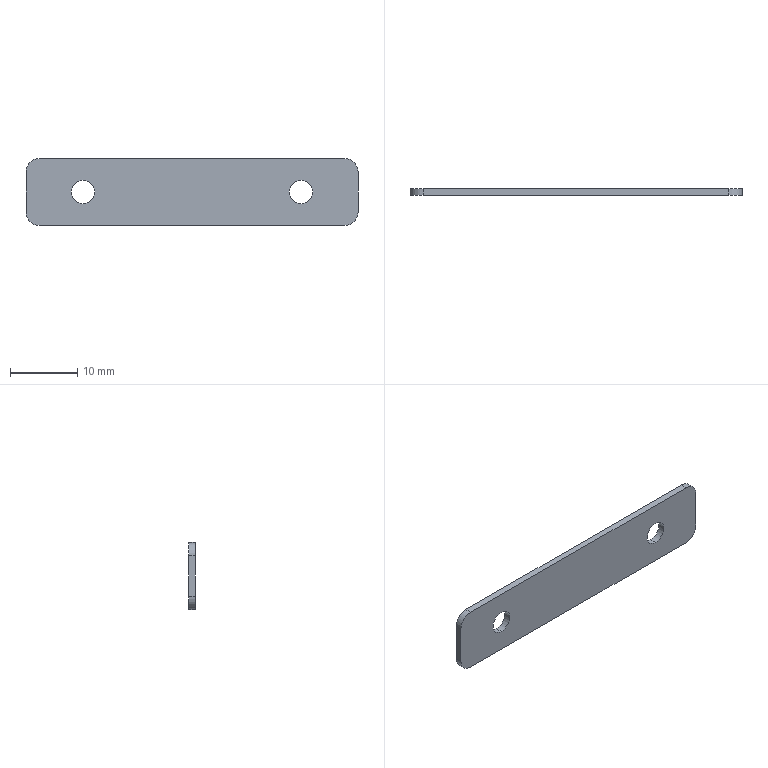Part | STEP file | 1 solid | 14 faces | box 49.5 x 1 x 10 mm | volume 472.324 mm3 | cylinder 8 | plane 6 | commonest cylinder face diameters 3.5 x4 4 x4
STEP:
#1=CARTESIAN_POINT('',(0.,0.,0.));
#2=DIRECTION('',(0.,0.,1.));
#3=DIRECTION('',(1.,0.,0.));
#4=AXIS2_PLACEMENT_3D('',#1,#2,#3);
#5=CARTESIAN_POINT('',(-16.25,1.,-1.75));
#6=VERTEX_POINT('',#5);
#7=CARTESIAN_POINT('',(-16.25,0.,-1.75));
#8=VERTEX_POINT('',#7);
#9=CARTESIAN_POINT('',(-16.25,1.,-1.75));
#10=DIRECTION('',(0.,-1.,0.));
#11=VECTOR('',#10,1.);
#12=LINE('',#9,#11);
#13=CARTESIAN_POINT('',(-16.25,1.,0.));
#14=DIRECTION('',(0.,-1.,0.));
#15=DIRECTION('',(0.,0.,-1.));
#16=AXIS2_PLACEMENT_3D('',#13,#14,#15);
#17=CYLINDRICAL_SURFACE('',#16,1.75);
#18=CARTESIAN_POINT('',(6.283,0.));
#19=DIRECTION('',(0.,1.));
#20=VECTOR('',#19,1.);
#21=LINE('',#18,#20);
#22=(GEOMETRIC_REPRESENTATION_CONTEXT(2)PARAMETRIC_REPRESENTATION_CONTEXT()REPRESENTATION_CONTEXT('',''));
#23=DEFINITIONAL_REPRESENTATION('',(#21),#22);
#24=PCURVE('',#17,#23);
#25=CARTESIAN_POINT('',(-16.25,1.,0.));
#26=DIRECTION('',(0.,-1.,0.));
#27=DIRECTION('',(0.,0.,-1.));
#28=AXIS2_PLACEMENT_3D('',#25,#26,#27);
#29=CYLINDRICAL_SURFACE('',#28,1.75);
#30=CARTESIAN_POINT('',(0.,0.));
#31=DIRECTION('',(0.,1.));
#32=VECTOR('',#31,1.);
#33=LINE('',#30,#32);
#34=(GEOMETRIC_REPRESENTATION_CONTEXT(2)PARAMETRIC_REPRESENTATION_CONTEXT()REPRESENTATION_CONTEXT('',''));
#35=DEFINITIONAL_REPRESENTATION('',(#33),#34);
#36=PCURVE('',#29,#35);
#37=SURFACE_CURVE('',#12,(#24,#36),.PCURVE_S1.);
#38=EDGE_CURVE('',#6,#8,#37,.T.);
#39=ORIENTED_EDGE('',*,*,#38,.T.);
#40=CARTESIAN_POINT('',(-16.25,0.,1.75));
#41=VERTEX_POINT('',#40);
#42=CARTESIAN_POINT('',(-16.25,0.,0.));
#43=DIRECTION('',(0.,1.,0.));
#44=DIRECTION('',(0.,0.,-1.));
#45=AXIS2_PLACEMENT_3D('',#42,#43,#44);
#46=CIRCLE('',#45,1.75);
#47=CARTESIAN_POINT('',(6.283,1.));
#48=DIRECTION('',(-1.,0.));
#49=VECTOR('',#48,1.);
#50=LINE('',#47,#49);
#51=(GEOMETRIC_REPRESENTATION_CONTEXT(2)PARAMETRIC_REPRESENTATION_CONTEXT()REPRESENTATION_CONTEXT('',''));
#52=DEFINITIONAL_REPRESENTATION('',(#50),#51);
#53=PCURVE('',#17,#52);
#54=CARTESIAN_POINT('',(0.,0.,0.));
#55=DIRECTION('',(0.,1.,0.));
#56=DIRECTION('',(1.,0.,0.));
#57=AXIS2_PLACEMENT_3D('',#54,#55,#56);
#58=PLANE('',#57);
#59=CARTESIAN_POINT('',(-16.25,0.));
#60=DIRECTION('',(0.,1.));
#61=AXIS2_PLACEMENT_2D('',#59,#60);
#62=CIRCLE('',#61,1.75);
#63=(GEOMETRIC_REPRESENTATION_CONTEXT(2)PARAMETRIC_REPRESENTATION_CONTEXT()REPRESENTATION_CONTEXT('',''));
#64=DEFINITIONAL_REPRESENTATION('',(#62),#63);
#65=PCURVE('',#58,#64);
#66=SURFACE_CURVE('',#46,(#53,#65),.PCURVE_S1.);
#67=EDGE_CURVE('',#8,#41,#66,.T.);
#68=ORIENTED_EDGE('',*,*,#67,.T.);
#69=CARTESIAN_POINT('',(-16.25,1.,1.75));
#70=VERTEX_POINT('',#69);
#71=CARTESIAN_POINT('',(-16.25,1.,1.75));
#72=DIRECTION('',(0.,-1.,0.));
#73=VECTOR('',#72,1.);
#74=LINE('',#71,#73);
#75=CARTESIAN_POINT('',(3.142,0.));
#76=DIRECTION('',(0.,1.));
#77=VECTOR('',#76,1.);
#78=LINE('',#75,#77);
#79=(GEOMETRIC_REPRESENTATION_CONTEXT(2)PARAMETRIC_REPRESENTATION_CONTEXT()REPRESENTATION_CONTEXT('',''));
#80=DEFINITIONAL_REPRESENTATION('',(#78),#79);
#81=PCURVE('',#17,#80);
#82=CARTESIAN_POINT('',(3.142,0.));
#83=DIRECTION('',(0.,1.));
#84=VECTOR('',#83,1.);
#85=LINE('',#82,#84);
#86=(GEOMETRIC_REPRESENTATION_CONTEXT(2)PARAMETRIC_REPRESENTATION_CONTEXT()REPRESENTATION_CONTEXT('',''));
#87=DEFINITIONAL_REPRESENTATION('',(#85),#86);
#88=PCURVE('',#29,#87);
#89=SURFACE_CURVE('',#74,(#81,#88),.PCURVE_S1.);
#90=EDGE_CURVE('',#70,#41,#89,.T.);
#91=ORIENTED_EDGE('',*,*,#90,.F.);
#92=CARTESIAN_POINT('',(-16.25,1.,0.));
#93=DIRECTION('',(0.,-1.,0.));
#94=DIRECTION('',(0.,0.,-1.));
#95=AXIS2_PLACEMENT_3D('',#92,#93,#94);
#96=CIRCLE('',#95,1.75);
#97=CARTESIAN_POINT('',(0.,0.));
#98=DIRECTION('',(1.,0.));
#99=VECTOR('',#98,1.);
#100=LINE('',#97,#99);
#101=(GEOMETRIC_REPRESENTATION_CONTEXT(2)PARAMETRIC_REPRESENTATION_CONTEXT()REPRESENTATION_CONTEXT('',''));
#102=DEFINITIONAL_REPRESENTATION('',(#100),#101);
#103=PCURVE('',#17,#102);
#104=CARTESIAN_POINT('',(0.,1.,0.));
#105=DIRECTION('',(0.,1.,0.));
#106=DIRECTION('',(1.,0.,0.));
#107=AXIS2_PLACEMENT_3D('',#104,#105,#106);
#108=PLANE('',#107);
#109=CARTESIAN_POINT('',(-16.25,1.75));
#110=CARTESIAN_POINT('',(-13.219,1.75));
#111=CARTESIAN_POINT('',(-14.734,-0.875));
#112=CARTESIAN_POINT('',(-16.25,-3.5));
#113=CARTESIAN_POINT('',(-17.766,-0.875));
#114=CARTESIAN_POINT('',(-19.281,1.75));
#115=CARTESIAN_POINT('',(-16.25,1.75));
#116=(BOUNDED_CURVE()B_SPLINE_CURVE(2,(#109,#110,#111,#112,#113,#114,#115),.UNSPECIFIED.,.T.,.F.)B_SPLINE_CURVE_WITH_KNOTS((1,2,2,2,2,1),(-2.094,0.,2.094,4.189,6.283,8.378),.UNSPECIFIED.)CURVE()GEOMETRIC_REPRESENTATION_ITEM()RATIONAL_B_SPLINE_CURVE((1.,0.5,1.,0.5,1.,0.5,1.))REPRESENTATION_ITEM(''));
#117=(GEOMETRIC_REPRESENTATION_CONTEXT(2)PARAMETRIC_REPRESENTATION_CONTEXT()REPRESENTATION_CONTEXT('',''));
#118=DEFINITIONAL_REPRESENTATION('',(#116),#117);
#119=PCURVE('',#108,#118);
#120=SURFACE_CURVE('',#96,(#103,#119),.PCURVE_S1.);
#121=EDGE_CURVE('',#70,#6,#120,.T.);
#122=ORIENTED_EDGE('',*,*,#121,.T.);
#123=EDGE_LOOP('',(#39,#68,#91,#122));
#124=FACE_BOUND('',#123,.F.);
#125=ADVANCED_FACE('',(#124),#17,.F.);
#126=CARTESIAN_POINT('',(16.25,1.,-1.75));
#127=VERTEX_POINT('',#126);
#128=CARTESIAN_POINT('',(16.25,0.,-1.75));
#129=VERTEX_POINT('',#128);
#130=CARTESIAN_POINT('',(16.25,1.,-1.75));
#131=DIRECTION('',(0.,-1.,0.));
#132=VECTOR('',#131,1.);
#133=LINE('',#130,#132);
#134=CARTESIAN_POINT('',(16.25,1.,0.));
#135=DIRECTION('',(0.,-1.,0.));
#136=DIRECTION('',(0.,0.,-1.));
#137=AXIS2_PLACEMENT_3D('',#134,#135,#136);
#138=CYLINDRICAL_SURFACE('',#137,1.75);
#139=CARTESIAN_POINT('',(6.283,0.));
#140=DIRECTION('',(0.,1.));
#141=VECTOR('',#140,1.);
#142=LINE('',#139,#141);
#143=(GEOMETRIC_REPRESENTATION_CONTEXT(2)PARAMETRIC_REPRESENTATION_CONTEXT()REPRESENTATION_CONTEXT('',''));
#144=DEFINITIONAL_REPRESENTATION('',(#142),#143);
#145=PCURVE('',#138,#144);
#146=CARTESIAN_POINT('',(16.25,1.,0.));
#147=DIRECTION('',(0.,-1.,0.));
#148=DIRECTION('',(0.,0.,-1.));
#149=AXIS2_PLACEMENT_3D('',#146,#147,#148);
#150=CYLINDRICAL_SURFACE('',#149,1.75);
#151=CARTESIAN_POINT('',(0.,0.));
#152=DIRECTION('',(0.,1.));
#153=VECTOR('',#152,1.);
#154=LINE('',#151,#153);
#155=(GEOMETRIC_REPRESENTATION_CONTEXT(2)PARAMETRIC_REPRESENTATION_CONTEXT()REPRESENTATION_CONTEXT('',''));
#156=DEFINITIONAL_REPRESENTATION('',(#154),#155);
#157=PCURVE('',#150,#156);
#158=SURFACE_CURVE('',#133,(#145,#157),.PCURVE_S1.);
#159=EDGE_CURVE('',#127,#129,#158,.T.);
#160=ORIENTED_EDGE('',*,*,#159,.T.);
#161=CARTESIAN_POINT('',(16.25,0.,1.75));
#162=VERTEX_POINT('',#161);
#163=CARTESIAN_POINT('',(16.25,0.,0.));
#164=DIRECTION('',(0.,1.,0.));
#165=DIRECTION('',(0.,0.,-1.));
#166=AXIS2_PLACEMENT_3D('',#163,#164,#165);
#167=CIRCLE('',#166,1.75);
#168=CARTESIAN_POINT('',(6.283,1.));
#169=DIRECTION('',(-1.,0.));
#170=VECTOR('',#169,1.);
#171=LINE('',#168,#170);
#172=(GEOMETRIC_REPRESENTATION_CONTEXT(2)PARAMETRIC_REPRESENTATION_CONTEXT()REPRESENTATION_CONTEXT('',''));
#173=DEFINITIONAL_REPRESENTATION('',(#171),#172);
#174=PCURVE('',#138,#173);
#175=CARTESIAN_POINT('',(16.25,0.));
#176=DIRECTION('',(0.,1.));
#177=AXIS2_PLACEMENT_2D('',#175,#176);
#178=CIRCLE('',#177,1.75);
#179=(GEOMETRIC_REPRESENTATION_CONTEXT(2)PARAMETRIC_REPRESENTATION_CONTEXT()REPRESENTATION_CONTEXT('',''));
#180=DEFINITIONAL_REPRESENTATION('',(#178),#179);
#181=PCURVE('',#58,#180);
#182=SURFACE_CURVE('',#167,(#174,#181),.PCURVE_S1.);
#183=EDGE_CURVE('',#129,#162,#182,.T.);
#184=ORIENTED_EDGE('',*,*,#183,.T.);
#185=CARTESIAN_POINT('',(16.25,1.,1.75));
#186=VERTEX_POINT('',#185);
#187=CARTESIAN_POINT('',(16.25,1.,1.75));
#188=DIRECTION('',(0.,-1.,0.));
#189=VECTOR('',#188,1.);
#190=LINE('',#187,#189);
#191=CARTESIAN_POINT('',(3.142,0.));
#192=DIRECTION('',(0.,1.));
#193=VECTOR('',#192,1.);
#194=LINE('',#191,#193);
#195=(GEOMETRIC_REPRESENTATION_CONTEXT(2)PARAMETRIC_REPRESENTATION_CONTEXT()REPRESENTATION_CONTEXT('',''));
#196=DEFINITIONAL_REPRESENTATION('',(#194),#195);
#197=PCURVE('',#138,#196);
#198=CARTESIAN_POINT('',(3.142,0.));
#199=DIRECTION('',(0.,1.));
#200=VECTOR('',#199,1.);
#201=LINE('',#198,#200);
#202=(GEOMETRIC_REPRESENTATION_CONTEXT(2)PARAMETRIC_REPRESENTATION_CONTEXT()REPRESENTATION_CONTEXT('',''));
#203=DEFINITIONAL_REPRESENTATION('',(#201),#202);
#204=PCURVE('',#150,#203);
#205=SURFACE_CURVE('',#190,(#197,#204),.PCURVE_S1.);
#206=EDGE_CURVE('',#186,#162,#205,.T.);
#207=ORIENTED_EDGE('',*,*,#206,.F.);
#208=CARTESIAN_POINT('',(16.25,1.,0.));
#209=DIRECTION('',(0.,-1.,0.));
#210=DIRECTION('',(0.,0.,-1.));
#211=AXIS2_PLACEMENT_3D('',#208,#209,#210);
#212=CIRCLE('',#211,1.75);
#213=CARTESIAN_POINT('',(0.,0.));
#214=DIRECTION('',(1.,0.));
#215=VECTOR('',#214,1.);
#216=LINE('',#213,#215);
#217=(GEOMETRIC_REPRESENTATION_CONTEXT(2)PARAMETRIC_REPRESENTATION_CONTEXT()REPRESENTATION_CONTEXT('',''));
#218=DEFINITIONAL_REPRESENTATION('',(#216),#217);
#219=PCURVE('',#138,#218);
#220=CARTESIAN_POINT('',(16.25,1.75));
#221=CARTESIAN_POINT('',(19.281,1.75));
#222=CARTESIAN_POINT('',(17.766,-0.875));
#223=CARTESIAN_POINT('',(16.25,-3.5));
#224=CARTESIAN_POINT('',(14.734,-0.875));
#225=CARTESIAN_POINT('',(13.219,1.75));
#226=CARTESIAN_POINT('',(16.25,1.75));
#227=(BOUNDED_CURVE()B_SPLINE_CURVE(2,(#220,#221,#222,#223,#224,#225,#226),.UNSPECIFIED.,.T.,.F.)B_SPLINE_CURVE_WITH_KNOTS((1,2,2,2,2,1),(-2.094,0.,2.094,4.189,6.283,8.378),.UNSPECIFIED.)CURVE()GEOMETRIC_REPRESENTATION_ITEM()RATIONAL_B_SPLINE_CURVE((1.,0.5,1.,0.5,1.,0.5,1.))REPRESENTATION_ITEM(''));
#228=(GEOMETRIC_REPRESENTATION_CONTEXT(2)PARAMETRIC_REPRESENTATION_CONTEXT()REPRESENTATION_CONTEXT('',''));
#229=DEFINITIONAL_REPRESENTATION('',(#227),#228);
#230=PCURVE('',#108,#229);
#231=SURFACE_CURVE('',#212,(#219,#230),.PCURVE_S1.);
#232=EDGE_CURVE('',#186,#127,#231,.T.);
#233=ORIENTED_EDGE('',*,*,#232,.T.);
#234=EDGE_LOOP('',(#160,#184,#207,#233));
#235=FACE_BOUND('',#234,.F.);
#236=ADVANCED_FACE('',(#235),#138,.F.);
#237=CARTESIAN_POINT('',(-22.75,1.,5.));
#238=VERTEX_POINT('',#237);
#239=CARTESIAN_POINT('',(22.75,1.,5.));
#240=VERTEX_POINT('',#239);
#241=CARTESIAN_POINT('',(0.,1.,5.));
#242=DIRECTION('',(1.,0.,0.));
#243=VECTOR('',#242,1.);
#244=LINE('',#241,#243);
#245=CARTESIAN_POINT('',(0.,-5.));
#246=DIRECTION('',(1.,0.));
#247=VECTOR('',#246,1.);
#248=LINE('',#245,#247);
#249=(GEOMETRIC_REPRESENTATION_CONTEXT(2)PARAMETRIC_REPRESENTATION_CONTEXT()REPRESENTATION_CONTEXT('',''));
#250=DEFINITIONAL_REPRESENTATION('',(#248),#249);
#251=PCURVE('',#108,#250);
#252=CARTESIAN_POINT('',(-24.75,1.,5.));
#253=DIRECTION('',(0.,0.,-1.));
#254=DIRECTION('',(0.,-1.,0.));
#255=AXIS2_PLACEMENT_3D('',#252,#253,#254);
#256=PLANE('',#255);
#257=CARTESIAN_POINT('',(0.,-24.75));
#258=DIRECTION('',(0.,-1.));
#259=VECTOR('',#258,1.);
#260=LINE('',#257,#259);
#261=(GEOMETRIC_REPRESENTATION_CONTEXT(2)PARAMETRIC_REPRESENTATION_CONTEXT()REPRESENTATION_CONTEXT('',''));
#262=DEFINITIONAL_REPRESENTATION('',(#260),#261);
#263=PCURVE('',#256,#262);
#264=SURFACE_CURVE('',#244,(#251,#263),.PCURVE_S1.);
#265=EDGE_CURVE('',#238,#240,#264,.T.);
#266=ORIENTED_EDGE('',*,*,#265,.T.);
#267=CARTESIAN_POINT('',(24.75,1.,3.));
#268=VERTEX_POINT('',#267);
#269=CARTESIAN_POINT('',(22.75,1.,3.));
#270=DIRECTION('',(0.,1.,0.));
#271=DIRECTION('',(0.,0.,-1.));
#272=AXIS2_PLACEMENT_3D('',#269,#270,#271);
#273=CIRCLE('',#272,2.);
#274=CARTESIAN_POINT('',(22.75,-3.));
#275=DIRECTION('',(0.,1.));
#276=AXIS2_PLACEMENT_2D('',#274,#275);
#277=CIRCLE('',#276,2.);
#278=(GEOMETRIC_REPRESENTATION_CONTEXT(2)PARAMETRIC_REPRESENTATION_CONTEXT()REPRESENTATION_CONTEXT('',''));
#279=DEFINITIONAL_REPRESENTATION('',(#277),#278);
#280=PCURVE('',#108,#279);
#281=CARTESIAN_POINT('',(22.75,1.,3.));
#282=DIRECTION('',(0.,-1.,0.));
#283=DIRECTION('',(0.,0.,-1.));
#284=AXIS2_PLACEMENT_3D('',#281,#282,#283);
#285=CYLINDRICAL_SURFACE('',#284,2.);
#286=CARTESIAN_POINT('',(6.283,0.));
#287=DIRECTION('',(-1.,0.));
#288=VECTOR('',#287,1.);
#289=LINE('',#286,#288);
#290=(GEOMETRIC_REPRESENTATION_CONTEXT(2)PARAMETRIC_REPRESENTATION_CONTEXT()REPRESENTATION_CONTEXT('',''));
#291=DEFINITIONAL_REPRESENTATION('',(#289),#290);
#292=PCURVE('',#285,#291);
#293=SURFACE_CURVE('',#273,(#280,#292),.PCURVE_S1.);
#294=EDGE_CURVE('',#240,#268,#293,.T.);
#295=ORIENTED_EDGE('',*,*,#294,.T.);
#296=CARTESIAN_POINT('',(24.75,1.,-3.));
#297=VERTEX_POINT('',#296);
#298=CARTESIAN_POINT('',(24.75,1.,0.));
#299=DIRECTION('',(0.,0.,-1.));
#300=VECTOR('',#299,1.);
#301=LINE('',#298,#300);
#302=CARTESIAN_POINT('',(24.75,0.));
#303=DIRECTION('',(0.,1.));
#304=VECTOR('',#303,1.);
#305=LINE('',#302,#304);
#306=(GEOMETRIC_REPRESENTATION_CONTEXT(2)PARAMETRIC_REPRESENTATION_CONTEXT()REPRESENTATION_CONTEXT('',''));
#307=DEFINITIONAL_REPRESENTATION('',(#305),#306);
#308=PCURVE('',#108,#307);
#309=CARTESIAN_POINT('',(24.75,1.,-5.));
#310=DIRECTION('',(-1.,0.,0.));
#311=DIRECTION('',(0.,1.,0.));
#312=AXIS2_PLACEMENT_3D('',#309,#310,#311);
#313=PLANE('',#312);
#314=CARTESIAN_POINT('',(0.,-5.));
#315=DIRECTION('',(0.,1.));
#316=VECTOR('',#315,1.);
#317=LINE('',#314,#316);
#318=(GEOMETRIC_REPRESENTATION_CONTEXT(2)PARAMETRIC_REPRESENTATION_CONTEXT()REPRESENTATION_CONTEXT('',''));
#319=DEFINITIONAL_REPRESENTATION('',(#317),#318);
#320=PCURVE('',#313,#319);
#321=SURFACE_CURVE('',#301,(#308,#320),.PCURVE_S1.);
#322=EDGE_CURVE('',#268,#297,#321,.T.);
#323=ORIENTED_EDGE('',*,*,#322,.T.);
#324=CARTESIAN_POINT('',(22.75,1.,-5.));
#325=VERTEX_POINT('',#324);
#326=CARTESIAN_POINT('',(22.75,1.,-3.));
#327=DIRECTION('',(0.,1.,0.));
#328=DIRECTION('',(0.,0.,-1.));
#329=AXIS2_PLACEMENT_3D('',#326,#327,#328);
#330=CIRCLE('',#329,2.);
#331=CARTESIAN_POINT('',(22.75,3.));
#332=DIRECTION('',(0.,1.));
#333=AXIS2_PLACEMENT_2D('',#331,#332);
#334=CIRCLE('',#333,2.);
#335=(GEOMETRIC_REPRESENTATION_CONTEXT(2)PARAMETRIC_REPRESENTATION_CONTEXT()REPRESENTATION_CONTEXT('',''));
#336=DEFINITIONAL_REPRESENTATION('',(#334),#335);
#337=PCURVE('',#108,#336);
#338=CARTESIAN_POINT('',(22.75,1.,-3.));
#339=DIRECTION('',(0.,-1.,0.));
#340=DIRECTION('',(0.,0.,-1.));
#341=AXIS2_PLACEMENT_3D('',#338,#339,#340);
#342=CYLINDRICAL_SURFACE('',#341,2.);
#343=CARTESIAN_POINT('',(6.283,0.));
#344=DIRECTION('',(-1.,0.));
#345=VECTOR('',#344,1.);
#346=LINE('',#343,#345);
#347=(GEOMETRIC_REPRESENTATION_CONTEXT(2)PARAMETRIC_REPRESENTATION_CONTEXT()REPRESENTATION_CONTEXT('',''));
#348=DEFINITIONAL_REPRESENTATION('',(#346),#347);
#349=PCURVE('',#342,#348);
#350=SURFACE_CURVE('',#330,(#337,#349),.PCURVE_S1.);
#351=EDGE_CURVE('',#297,#325,#350,.T.);
#352=ORIENTED_EDGE('',*,*,#351,.T.);
#353=CARTESIAN_POINT('',(-22.75,1.,-5.));
#354=VERTEX_POINT('',#353);
#355=CARTESIAN_POINT('',(0.,1.,-5.));
#356=DIRECTION('',(-1.,0.,0.));
#357=VECTOR('',#356,1.);
#358=LINE('',#355,#357);
#359=CARTESIAN_POINT('',(0.,5.));
#360=DIRECTION('',(-1.,0.));
#361=VECTOR('',#360,1.);
#362=LINE('',#359,#361);
#363=(GEOMETRIC_REPRESENTATION_CONTEXT(2)PARAMETRIC_REPRESENTATION_CONTEXT()REPRESENTATION_CONTEXT('',''));
#364=DEFINITIONAL_REPRESENTATION('',(#362),#363);
#365=PCURVE('',#108,#364);
#366=CARTESIAN_POINT('',(-24.75,1.,-5.));
#367=DIRECTION('',(0.,0.,1.));
#368=DIRECTION('',(1.,0.,0.));
#369=AXIS2_PLACEMENT_3D('',#366,#367,#368);
#370=PLANE('',#369);
#371=CARTESIAN_POINT('',(24.75,0.));
#372=DIRECTION('',(-1.,0.));
#373=VECTOR('',#372,1.);
#374=LINE('',#371,#373);
#375=(GEOMETRIC_REPRESENTATION_CONTEXT(2)PARAMETRIC_REPRESENTATION_CONTEXT()REPRESENTATION_CONTEXT('',''));
#376=DEFINITIONAL_REPRESENTATION('',(#374),#375);
#377=PCURVE('',#370,#376);
#378=SURFACE_CURVE('',#358,(#365,#377),.PCURVE_S1.);
#379=EDGE_CURVE('',#325,#354,#378,.T.);
#380=ORIENTED_EDGE('',*,*,#379,.T.);
#381=CARTESIAN_POINT('',(-24.75,1.,-3.));
#382=VERTEX_POINT('',#381);
#383=CARTESIAN_POINT('',(-22.75,1.,-3.));
#384=DIRECTION('',(0.,1.,0.));
#385=DIRECTION('',(0.,0.,-1.));
#386=AXIS2_PLACEMENT_3D('',#383,#384,#385);
#387=CIRCLE('',#386,2.);
#388=CARTESIAN_POINT('',(-22.75,3.));
#389=DIRECTION('',(0.,1.));
#390=AXIS2_PLACEMENT_2D('',#388,#389);
#391=CIRCLE('',#390,2.);
#392=(GEOMETRIC_REPRESENTATION_CONTEXT(2)PARAMETRIC_REPRESENTATION_CONTEXT()REPRESENTATION_CONTEXT('',''));
#393=DEFINITIONAL_REPRESENTATION('',(#391),#392);
#394=PCURVE('',#108,#393);
#395=CARTESIAN_POINT('',(-22.75,1.,-3.));
#396=DIRECTION('',(0.,-1.,0.));
#397=DIRECTION('',(0.,0.,-1.));
#398=AXIS2_PLACEMENT_3D('',#395,#396,#397);
#399=CYLINDRICAL_SURFACE('',#398,2.);
#400=CARTESIAN_POINT('',(6.283,0.));
#401=DIRECTION('',(-1.,0.));
#402=VECTOR('',#401,1.);
#403=LINE('',#400,#402);
#404=(GEOMETRIC_REPRESENTATION_CONTEXT(2)PARAMETRIC_REPRESENTATION_CONTEXT()REPRESENTATION_CONTEXT('',''));
#405=DEFINITIONAL_REPRESENTATION('',(#403),#404);
#406=PCURVE('',#399,#405);
#407=SURFACE_CURVE('',#387,(#394,#406),.PCURVE_S1.);
#408=EDGE_CURVE('',#354,#382,#407,.T.);
#409=ORIENTED_EDGE('',*,*,#408,.T.);
#410=CARTESIAN_POINT('',(-24.75,1.,3.));
#411=VERTEX_POINT('',#410);
#412=CARTESIAN_POINT('',(-24.75,1.,0.));
#413=DIRECTION('',(0.,0.,1.));
#414=VECTOR('',#413,1.);
#415=LINE('',#412,#414);
#416=CARTESIAN_POINT('',(-24.75,0.));
#417=DIRECTION('',(0.,-1.));
#418=VECTOR('',#417,1.);
#419=LINE('',#416,#418);
#420=(GEOMETRIC_REPRESENTATION_CONTEXT(2)PARAMETRIC_REPRESENTATION_CONTEXT()REPRESENTATION_CONTEXT('',''));
#421=DEFINITIONAL_REPRESENTATION('',(#419),#420);
#422=PCURVE('',#108,#421);
#423=CARTESIAN_POINT('',(-24.75,1.,-5.));
#424=DIRECTION('',(1.,0.,0.));
#425=DIRECTION('',(0.,0.,1.));
#426=AXIS2_PLACEMENT_3D('',#423,#424,#425);
#427=PLANE('',#426);
#428=CARTESIAN_POINT('',(5.,0.));
#429=DIRECTION('',(1.,0.));
#430=VECTOR('',#429,1.);
#431=LINE('',#428,#430);
#432=(GEOMETRIC_REPRESENTATION_CONTEXT(2)PARAMETRIC_REPRESENTATION_CONTEXT()REPRESENTATION_CONTEXT('',''));
#433=DEFINITIONAL_REPRESENTATION('',(#431),#432);
#434=PCURVE('',#427,#433);
#435=SURFACE_CURVE('',#415,(#422,#434),.PCURVE_S1.);
#436=EDGE_CURVE('',#382,#411,#435,.T.);
#437=ORIENTED_EDGE('',*,*,#436,.T.);
#438=CARTESIAN_POINT('',(-22.75,1.,3.));
#439=DIRECTION('',(0.,1.,0.));
#440=DIRECTION('',(0.,0.,-1.));
#441=AXIS2_PLACEMENT_3D('',#438,#439,#440);
#442=CIRCLE('',#441,2.);
#443=CARTESIAN_POINT('',(-22.75,-3.));
#444=DIRECTION('',(0.,1.));
#445=AXIS2_PLACEMENT_2D('',#443,#444);
#446=CIRCLE('',#445,2.);
#447=(GEOMETRIC_REPRESENTATION_CONTEXT(2)PARAMETRIC_REPRESENTATION_CONTEXT()REPRESENTATION_CONTEXT('',''));
#448=DEFINITIONAL_REPRESENTATION('',(#446),#447);
#449=PCURVE('',#108,#448);
#450=CARTESIAN_POINT('',(-22.75,1.,3.));
#451=DIRECTION('',(0.,-1.,0.));
#452=DIRECTION('',(0.,0.,-1.));
#453=AXIS2_PLACEMENT_3D('',#450,#451,#452);
#454=CYLINDRICAL_SURFACE('',#453,2.);
#455=CARTESIAN_POINT('',(6.283,0.));
#456=DIRECTION('',(-1.,0.));
#457=VECTOR('',#456,1.);
#458=LINE('',#455,#457);
#459=(GEOMETRIC_REPRESENTATION_CONTEXT(2)PARAMETRIC_REPRESENTATION_CONTEXT()REPRESENTATION_CONTEXT('',''));
#460=DEFINITIONAL_REPRESENTATION('',(#458),#459);
#461=PCURVE('',#454,#460);
#462=SURFACE_CURVE('',#442,(#449,#461),.PCURVE_S1.);
#463=EDGE_CURVE('',#411,#238,#462,.T.);
#464=ORIENTED_EDGE('',*,*,#463,.T.);
#465=EDGE_LOOP('',(#266,#295,#323,#352,#380,#409,#437,#464));
#466=FACE_BOUND('',#465,.T.);
#467=CARTESIAN_POINT('',(-16.25,1.,0.));
#468=DIRECTION('',(0.,-1.,0.));
#469=DIRECTION('',(0.,0.,-1.));
#470=AXIS2_PLACEMENT_3D('',#467,#468,#469);
#471=CIRCLE('',#470,1.75);
#472=CARTESIAN_POINT('',(-16.25,1.75));
#473=CARTESIAN_POINT('',(-13.219,1.75));
#474=CARTESIAN_POINT('',(-14.734,-0.875));
#475=CARTESIAN_POINT('',(-16.25,-3.5));
#476=CARTESIAN_POINT('',(-17.766,-0.875));
#477=CARTESIAN_POINT('',(-19.281,1.75));
#478=CARTESIAN_POINT('',(-16.25,1.75));
#479=(BOUNDED_CURVE()B_SPLINE_CURVE(2,(#472,#473,#474,#475,#476,#477,#478),.UNSPECIFIED.,.T.,.F.)B_SPLINE_CURVE_WITH_KNOTS((1,2,2,2,2,1),(-2.094,0.,2.094,4.189,6.283,8.378),.UNSPECIFIED.)CURVE()GEOMETRIC_REPRESENTATION_ITEM()RATIONAL_B_SPLINE_CURVE((1.,0.5,1.,0.5,1.,0.5,1.))REPRESENTATION_ITEM(''));
#480=(GEOMETRIC_REPRESENTATION_CONTEXT(2)PARAMETRIC_REPRESENTATION_CONTEXT()REPRESENTATION_CONTEXT('',''));
#481=DEFINITIONAL_REPRESENTATION('',(#479),#480);
#482=PCURVE('',#108,#481);
#483=CARTESIAN_POINT('',(0.,0.));
#484=DIRECTION('',(1.,0.));
#485=VECTOR('',#484,1.);
#486=LINE('',#483,#485);
#487=(GEOMETRIC_REPRESENTATION_CONTEXT(2)PARAMETRIC_REPRESENTATION_CONTEXT()REPRESENTATION_CONTEXT('',''));
#488=DEFINITIONAL_REPRESENTATION('',(#486),#487);
#489=PCURVE('',#29,#488);
#490=SURFACE_CURVE('',#471,(#482,#489),.PCURVE_S1.);
#491=EDGE_CURVE('',#6,#70,#490,.T.);
#492=ORIENTED_EDGE('',*,*,#491,.T.);
#493=ORIENTED_EDGE('',*,*,#121,.T.);
#494=EDGE_LOOP('',(#492,#493));
#495=FACE_BOUND('',#494,.T.);
#496=CARTESIAN_POINT('',(16.25,1.,0.));
#497=DIRECTION('',(0.,-1.,0.));
#498=DIRECTION('',(0.,0.,-1.));
#499=AXIS2_PLACEMENT_3D('',#496,#497,#498);
#500=CIRCLE('',#499,1.75);
#501=CARTESIAN_POINT('',(16.25,1.75));
#502=CARTESIAN_POINT('',(19.281,1.75));
#503=CARTESIAN_POINT('',(17.766,-0.875));
#504=CARTESIAN_POINT('',(16.25,-3.5));
#505=CARTESIAN_POINT('',(14.734,-0.875));
#506=CARTESIAN_POINT('',(13.219,1.75));
#507=CARTESIAN_POINT('',(16.25,1.75));
#508=(BOUNDED_CURVE()B_SPLINE_CURVE(2,(#501,#502,#503,#504,#505,#506,#507),.UNSPECIFIED.,.T.,.F.)B_SPLINE_CURVE_WITH_KNOTS((1,2,2,2,2,1),(-2.094,0.,2.094,4.189,6.283,8.378),.UNSPECIFIED.)CURVE()GEOMETRIC_REPRESENTATION_ITEM()RATIONAL_B_SPLINE_CURVE((1.,0.5,1.,0.5,1.,0.5,1.))REPRESENTATION_ITEM(''));
#509=(GEOMETRIC_REPRESENTATION_CONTEXT(2)PARAMETRIC_REPRESENTATION_CONTEXT()REPRESENTATION_CONTEXT('',''));
#510=DEFINITIONAL_REPRESENTATION('',(#508),#509);
#511=PCURVE('',#108,#510);
#512=CARTESIAN_POINT('',(0.,0.));
#513=DIRECTION('',(1.,0.));
#514=VECTOR('',#513,1.);
#515=LINE('',#512,#514);
#516=(GEOMETRIC_REPRESENTATION_CONTEXT(2)PARAMETRIC_REPRESENTATION_CONTEXT()REPRESENTATION_CONTEXT('',''));
#517=DEFINITIONAL_REPRESENTATION('',(#515),#516);
#518=PCURVE('',#150,#517);
#519=SURFACE_CURVE('',#500,(#511,#518),.PCURVE_S1.);
#520=EDGE_CURVE('',#127,#186,#519,.T.);
#521=ORIENTED_EDGE('',*,*,#520,.T.);
#522=ORIENTED_EDGE('',*,*,#232,.T.);
#523=EDGE_LOOP('',(#521,#522));
#524=FACE_BOUND('',#523,.T.);
#525=ADVANCED_FACE('',(#466,#495,#524),#108,.T.);
#526=CARTESIAN_POINT('',(-16.25,0.,0.));
#527=DIRECTION('',(0.,1.,0.));
#528=DIRECTION('',(0.,0.,-1.));
#529=AXIS2_PLACEMENT_3D('',#526,#527,#528);
#530=CIRCLE('',#529,1.75);
#531=CARTESIAN_POINT('',(6.283,1.));
#532=DIRECTION('',(-1.,0.));
#533=VECTOR('',#532,1.);
#534=LINE('',#531,#533);
#535=(GEOMETRIC_REPRESENTATION_CONTEXT(2)PARAMETRIC_REPRESENTATION_CONTEXT()REPRESENTATION_CONTEXT('',''));
#536=DEFINITIONAL_REPRESENTATION('',(#534),#535);
#537=PCURVE('',#29,#536);
#538=CARTESIAN_POINT('',(-16.25,0.));
#539=DIRECTION('',(0.,1.));
#540=AXIS2_PLACEMENT_2D('',#538,#539);
#541=CIRCLE('',#540,1.75);
#542=(GEOMETRIC_REPRESENTATION_CONTEXT(2)PARAMETRIC_REPRESENTATION_CONTEXT()REPRESENTATION_CONTEXT('',''));
#543=DEFINITIONAL_REPRESENTATION('',(#541),#542);
#544=PCURVE('',#58,#543);
#545=SURFACE_CURVE('',#530,(#537,#544),.PCURVE_S1.);
#546=EDGE_CURVE('',#41,#8,#545,.T.);
#547=ORIENTED_EDGE('',*,*,#546,.T.);
#548=ORIENTED_EDGE('',*,*,#38,.F.);
#549=ORIENTED_EDGE('',*,*,#491,.T.);
#550=ORIENTED_EDGE('',*,*,#90,.T.);
#551=EDGE_LOOP('',(#547,#548,#549,#550));
#552=FACE_BOUND('',#551,.F.);
#553=ADVANCED_FACE('',(#552),#29,.F.);
#554=ORIENTED_EDGE('',*,*,#294,.F.);
#555=CARTESIAN_POINT('',(22.75,0.,5.));
#556=VERTEX_POINT('',#555);
#557=CARTESIAN_POINT('',(22.75,1.,5.));
#558=DIRECTION('',(0.,-1.,0.));
#559=VECTOR('',#558,1.);
#560=LINE('',#557,#559);
#561=CARTESIAN_POINT('',(3.142,0.));
#562=DIRECTION('',(0.,1.));
#563=VECTOR('',#562,1.);
#564=LINE('',#561,#563);
#565=(GEOMETRIC_REPRESENTATION_CONTEXT(2)PARAMETRIC_REPRESENTATION_CONTEXT()REPRESENTATION_CONTEXT('',''));
#566=DEFINITIONAL_REPRESENTATION('',(#564),#565);
#567=PCURVE('',#285,#566);
#568=CARTESIAN_POINT('',(0.,-47.5));
#569=DIRECTION('',(1.,0.));
#570=VECTOR('',#569,1.);
#571=LINE('',#568,#570);
#572=(GEOMETRIC_REPRESENTATION_CONTEXT(2)PARAMETRIC_REPRESENTATION_CONTEXT()REPRESENTATION_CONTEXT('',''));
#573=DEFINITIONAL_REPRESENTATION('',(#571),#572);
#574=PCURVE('',#256,#573);
#575=SURFACE_CURVE('',#560,(#567,#574),.PCURVE_S1.);
#576=EDGE_CURVE('',#240,#556,#575,.T.);
#577=ORIENTED_EDGE('',*,*,#576,.T.);
#578=CARTESIAN_POINT('',(24.75,0.,3.));
#579=VERTEX_POINT('',#578);
#580=CARTESIAN_POINT('',(22.75,0.,3.));
#581=DIRECTION('',(0.,1.,0.));
#582=DIRECTION('',(0.,0.,-1.));
#583=AXIS2_PLACEMENT_3D('',#580,#581,#582);
#584=CIRCLE('',#583,2.);
#585=CARTESIAN_POINT('',(6.283,1.));
#586=DIRECTION('',(-1.,0.));
#587=VECTOR('',#586,1.);
#588=LINE('',#585,#587);
#589=(GEOMETRIC_REPRESENTATION_CONTEXT(2)PARAMETRIC_REPRESENTATION_CONTEXT()REPRESENTATION_CONTEXT('',''));
#590=DEFINITIONAL_REPRESENTATION('',(#588),#589);
#591=PCURVE('',#285,#590);
#592=CARTESIAN_POINT('',(22.75,-3.));
#593=DIRECTION('',(0.,1.));
#594=AXIS2_PLACEMENT_2D('',#592,#593);
#595=CIRCLE('',#594,2.);
#596=(GEOMETRIC_REPRESENTATION_CONTEXT(2)PARAMETRIC_REPRESENTATION_CONTEXT()REPRESENTATION_CONTEXT('',''));
#597=DEFINITIONAL_REPRESENTATION('',(#595),#596);
#598=PCURVE('',#58,#597);
#599=SURFACE_CURVE('',#584,(#591,#598),.PCURVE_S1.);
#600=EDGE_CURVE('',#556,#579,#599,.T.);
#601=ORIENTED_EDGE('',*,*,#600,.T.);
#602=CARTESIAN_POINT('',(24.75,1.,3.));
#603=DIRECTION('',(0.,1.,0.));
#604=VECTOR('',#603,1.);
#605=LINE('',#602,#604);
#606=CARTESIAN_POINT('',(1.571,0.));
#607=DIRECTION('',(0.,-1.));
#608=VECTOR('',#607,1.);
#609=LINE('',#606,#608);
#610=(GEOMETRIC_REPRESENTATION_CONTEXT(2)PARAMETRIC_REPRESENTATION_CONTEXT()REPRESENTATION_CONTEXT('',''));
#611=DEFINITIONAL_REPRESENTATION('',(#609),#610);
#612=PCURVE('',#285,#611);
#613=CARTESIAN_POINT('',(0.,-8.));
#614=DIRECTION('',(1.,0.));
#615=VECTOR('',#614,1.);
#616=LINE('',#613,#615);
#617=(GEOMETRIC_REPRESENTATION_CONTEXT(2)PARAMETRIC_REPRESENTATION_CONTEXT()REPRESENTATION_CONTEXT('',''));
#618=DEFINITIONAL_REPRESENTATION('',(#616),#617);
#619=PCURVE('',#313,#618);
#620=SURFACE_CURVE('',#605,(#612,#619),.PCURVE_S1.);
#621=EDGE_CURVE('',#579,#268,#620,.T.);
#622=ORIENTED_EDGE('',*,*,#621,.T.);
#623=EDGE_LOOP('',(#554,#577,#601,#622));
#624=FACE_BOUND('',#623,.T.);
#625=ADVANCED_FACE('',(#624),#285,.T.);
#626=CARTESIAN_POINT('',(-22.75,0.,5.));
#627=VERTEX_POINT('',#626);
#628=CARTESIAN_POINT('',(-24.75,0.,5.));
#629=DIRECTION('',(-1.,0.,0.));
#630=VECTOR('',#629,1.);
#631=LINE('',#628,#630);
#632=CARTESIAN_POINT('',(1.,0.));
#633=DIRECTION('',(0.,1.));
#634=VECTOR('',#633,1.);
#635=LINE('',#632,#634);
#636=(GEOMETRIC_REPRESENTATION_CONTEXT(2)PARAMETRIC_REPRESENTATION_CONTEXT()REPRESENTATION_CONTEXT('',''));
#637=DEFINITIONAL_REPRESENTATION('',(#635),#636);
#638=PCURVE('',#256,#637);
#639=CARTESIAN_POINT('',(-24.75,-5.));
#640=DIRECTION('',(-1.,0.));
#641=VECTOR('',#640,1.);
#642=LINE('',#639,#641);
#643=(GEOMETRIC_REPRESENTATION_CONTEXT(2)PARAMETRIC_REPRESENTATION_CONTEXT()REPRESENTATION_CONTEXT('',''));
#644=DEFINITIONAL_REPRESENTATION('',(#642),#643);
#645=PCURVE('',#58,#644);
#646=SURFACE_CURVE('',#631,(#638,#645),.PCURVE_S1.);
#647=EDGE_CURVE('',#556,#627,#646,.T.);
#648=ORIENTED_EDGE('',*,*,#647,.F.);
#649=ORIENTED_EDGE('',*,*,#576,.F.);
#650=ORIENTED_EDGE('',*,*,#265,.F.);
#651=CARTESIAN_POINT('',(-22.75,1.,5.));
#652=DIRECTION('',(0.,1.,0.));
#653=VECTOR('',#652,1.);
#654=LINE('',#651,#653);
#655=CARTESIAN_POINT('',(0.,-2.));
#656=DIRECTION('',(-1.,0.));
#657=VECTOR('',#656,1.);
#658=LINE('',#655,#657);
#659=(GEOMETRIC_REPRESENTATION_CONTEXT(2)PARAMETRIC_REPRESENTATION_CONTEXT()REPRESENTATION_CONTEXT('',''));
#660=DEFINITIONAL_REPRESENTATION('',(#658),#659);
#661=PCURVE('',#256,#660);
#662=CARTESIAN_POINT('',(3.142,0.));
#663=DIRECTION('',(0.,-1.));
#664=VECTOR('',#663,1.);
#665=LINE('',#662,#664);
#666=(GEOMETRIC_REPRESENTATION_CONTEXT(2)PARAMETRIC_REPRESENTATION_CONTEXT()REPRESENTATION_CONTEXT('',''));
#667=DEFINITIONAL_REPRESENTATION('',(#665),#666);
#668=PCURVE('',#454,#667);
#669=SURFACE_CURVE('',#654,(#661,#668),.PCURVE_S1.);
#670=EDGE_CURVE('',#627,#238,#669,.T.);
#671=ORIENTED_EDGE('',*,*,#670,.F.);
#672=EDGE_LOOP('',(#648,#649,#650,#671));
#673=FACE_BOUND('',#672,.T.);
#674=ADVANCED_FACE('',(#673),#256,.F.);
#675=ORIENTED_EDGE('',*,*,#463,.F.);
#676=CARTESIAN_POINT('',(-24.75,0.,3.));
#677=VERTEX_POINT('',#676);
#678=CARTESIAN_POINT('',(-24.75,1.,3.));
#679=DIRECTION('',(0.,-1.,0.));
#680=VECTOR('',#679,1.);
#681=LINE('',#678,#680);
#682=CARTESIAN_POINT('',(4.712,0.));
#683=DIRECTION('',(0.,1.));
#684=VECTOR('',#683,1.);
#685=LINE('',#682,#684);
#686=(GEOMETRIC_REPRESENTATION_CONTEXT(2)PARAMETRIC_REPRESENTATION_CONTEXT()REPRESENTATION_CONTEXT('',''));
#687=DEFINITIONAL_REPRESENTATION('',(#685),#686);
#688=PCURVE('',#454,#687);
#689=CARTESIAN_POINT('',(8.,0.));
#690=DIRECTION('',(0.,1.));
#691=VECTOR('',#690,1.);
#692=LINE('',#689,#691);
#693=(GEOMETRIC_REPRESENTATION_CONTEXT(2)PARAMETRIC_REPRESENTATION_CONTEXT()REPRESENTATION_CONTEXT('',''));
#694=DEFINITIONAL_REPRESENTATION('',(#692),#693);
#695=PCURVE('',#427,#694);
#696=SURFACE_CURVE('',#681,(#688,#695),.PCURVE_S1.);
#697=EDGE_CURVE('',#411,#677,#696,.T.);
#698=ORIENTED_EDGE('',*,*,#697,.T.);
#699=CARTESIAN_POINT('',(-22.75,0.,3.));
#700=DIRECTION('',(0.,1.,0.));
#701=DIRECTION('',(0.,0.,-1.));
#702=AXIS2_PLACEMENT_3D('',#699,#700,#701);
#703=CIRCLE('',#702,2.);
#704=CARTESIAN_POINT('',(6.283,1.));
#705=DIRECTION('',(-1.,0.));
#706=VECTOR('',#705,1.);
#707=LINE('',#704,#706);
#708=(GEOMETRIC_REPRESENTATION_CONTEXT(2)PARAMETRIC_REPRESENTATION_CONTEXT()REPRESENTATION_CONTEXT('',''));
#709=DEFINITIONAL_REPRESENTATION('',(#707),#708);
#710=PCURVE('',#454,#709);
#711=CARTESIAN_POINT('',(-22.75,-3.));
#712=DIRECTION('',(0.,1.));
#713=AXIS2_PLACEMENT_2D('',#711,#712);
#714=CIRCLE('',#713,2.);
#715=(GEOMETRIC_REPRESENTATION_CONTEXT(2)PARAMETRIC_REPRESENTATION_CONTEXT()REPRESENTATION_CONTEXT('',''));
#716=DEFINITIONAL_REPRESENTATION('',(#714),#715);
#717=PCURVE('',#58,#716);
#718=SURFACE_CURVE('',#703,(#710,#717),.PCURVE_S1.);
#719=EDGE_CURVE('',#677,#627,#718,.T.);
#720=ORIENTED_EDGE('',*,*,#719,.T.);
#721=ORIENTED_EDGE('',*,*,#670,.T.);
#722=EDGE_LOOP('',(#675,#698,#720,#721));
#723=FACE_BOUND('',#722,.T.);
#724=ADVANCED_FACE('',(#723),#454,.T.);
#725=CARTESIAN_POINT('',(-24.75,0.,-3.));
#726=VERTEX_POINT('',#725);
#727=CARTESIAN_POINT('',(-24.75,0.,-5.));
#728=DIRECTION('',(0.,0.,-1.));
#729=VECTOR('',#728,1.);
#730=LINE('',#727,#729);
#731=CARTESIAN_POINT('',(0.,1.));
#732=DIRECTION('',(-1.,0.));
#733=VECTOR('',#732,1.);
#734=LINE('',#731,#733);
#735=(GEOMETRIC_REPRESENTATION_CONTEXT(2)PARAMETRIC_REPRESENTATION_CONTEXT()REPRESENTATION_CONTEXT('',''));
#736=DEFINITIONAL_REPRESENTATION('',(#734),#735);
#737=PCURVE('',#427,#736);
#738=CARTESIAN_POINT('',(-24.75,5.));
#739=DIRECTION('',(0.,1.));
#740=VECTOR('',#739,1.);
#741=LINE('',#738,#740);
#742=(GEOMETRIC_REPRESENTATION_CONTEXT(2)PARAMETRIC_REPRESENTATION_CONTEXT()REPRESENTATION_CONTEXT('',''));
#743=DEFINITIONAL_REPRESENTATION('',(#741),#742);
#744=PCURVE('',#58,#743);
#745=SURFACE_CURVE('',#730,(#737,#744),.PCURVE_S1.);
#746=EDGE_CURVE('',#677,#726,#745,.T.);
#747=ORIENTED_EDGE('',*,*,#746,.F.);
#748=ORIENTED_EDGE('',*,*,#697,.F.);
#749=ORIENTED_EDGE('',*,*,#436,.F.);
#750=CARTESIAN_POINT('',(-24.75,1.,-3.));
#751=DIRECTION('',(0.,1.,0.));
#752=VECTOR('',#751,1.);
#753=LINE('',#750,#752);
#754=CARTESIAN_POINT('',(2.,0.));
#755=DIRECTION('',(0.,-1.));
#756=VECTOR('',#755,1.);
#757=LINE('',#754,#756);
#758=(GEOMETRIC_REPRESENTATION_CONTEXT(2)PARAMETRIC_REPRESENTATION_CONTEXT()REPRESENTATION_CONTEXT('',''));
#759=DEFINITIONAL_REPRESENTATION('',(#757),#758);
#760=PCURVE('',#427,#759);
#761=CARTESIAN_POINT('',(4.712,0.));
#762=DIRECTION('',(0.,-1.));
#763=VECTOR('',#762,1.);
#764=LINE('',#761,#763);
#765=(GEOMETRIC_REPRESENTATION_CONTEXT(2)PARAMETRIC_REPRESENTATION_CONTEXT()REPRESENTATION_CONTEXT('',''));
#766=DEFINITIONAL_REPRESENTATION('',(#764),#765);
#767=PCURVE('',#399,#766);
#768=SURFACE_CURVE('',#753,(#760,#767),.PCURVE_S1.);
#769=EDGE_CURVE('',#726,#382,#768,.T.);
#770=ORIENTED_EDGE('',*,*,#769,.F.);
#771=EDGE_LOOP('',(#747,#748,#749,#770));
#772=FACE_BOUND('',#771,.T.);
#773=ADVANCED_FACE('',(#772),#427,.F.);
#774=ORIENTED_EDGE('',*,*,#408,.F.);
#775=CARTESIAN_POINT('',(-22.75,0.,-5.));
#776=VERTEX_POINT('',#775);
#777=CARTESIAN_POINT('',(-22.75,1.,-5.));
#778=DIRECTION('',(0.,-1.,0.));
#779=VECTOR('',#778,1.);
#780=LINE('',#777,#779);
#781=CARTESIAN_POINT('',(6.283,0.));
#782=DIRECTION('',(0.,1.));
#783=VECTOR('',#782,1.);
#784=LINE('',#781,#783);
#785=(GEOMETRIC_REPRESENTATION_CONTEXT(2)PARAMETRIC_REPRESENTATION_CONTEXT()REPRESENTATION_CONTEXT('',''));
#786=DEFINITIONAL_REPRESENTATION('',(#784),#785);
#787=PCURVE('',#399,#786);
#788=CARTESIAN_POINT('',(2.,0.));
#789=DIRECTION('',(0.,-1.));
#790=VECTOR('',#789,1.);
#791=LINE('',#788,#790);
#792=(GEOMETRIC_REPRESENTATION_CONTEXT(2)PARAMETRIC_REPRESENTATION_CONTEXT()REPRESENTATION_CONTEXT('',''));
#793=DEFINITIONAL_REPRESENTATION('',(#791),#792);
#794=PCURVE('',#370,#793);
#795=SURFACE_CURVE('',#780,(#787,#794),.PCURVE_S1.);
#796=EDGE_CURVE('',#354,#776,#795,.T.);
#797=ORIENTED_EDGE('',*,*,#796,.T.);
#798=CARTESIAN_POINT('',(-22.75,0.,-3.));
#799=DIRECTION('',(0.,1.,0.));
#800=DIRECTION('',(0.,0.,-1.));
#801=AXIS2_PLACEMENT_3D('',#798,#799,#800);
#802=CIRCLE('',#801,2.);
#803=CARTESIAN_POINT('',(6.283,1.));
#804=DIRECTION('',(-1.,0.));
#805=VECTOR('',#804,1.);
#806=LINE('',#803,#805);
#807=(GEOMETRIC_REPRESENTATION_CONTEXT(2)PARAMETRIC_REPRESENTATION_CONTEXT()REPRESENTATION_CONTEXT('',''));
#808=DEFINITIONAL_REPRESENTATION('',(#806),#807);
#809=PCURVE('',#399,#808);
#810=CARTESIAN_POINT('',(-22.75,3.));
#811=DIRECTION('',(0.,1.));
#812=AXIS2_PLACEMENT_2D('',#810,#811);
#813=CIRCLE('',#812,2.);
#814=(GEOMETRIC_REPRESENTATION_CONTEXT(2)PARAMETRIC_REPRESENTATION_CONTEXT()REPRESENTATION_CONTEXT('',''));
#815=DEFINITIONAL_REPRESENTATION('',(#813),#814);
#816=PCURVE('',#58,#815);
#817=SURFACE_CURVE('',#802,(#809,#816),.PCURVE_S1.);
#818=EDGE_CURVE('',#776,#726,#817,.T.);
#819=ORIENTED_EDGE('',*,*,#818,.T.);
#820=ORIENTED_EDGE('',*,*,#769,.T.);
#821=EDGE_LOOP('',(#774,#797,#819,#820));
#822=FACE_BOUND('',#821,.T.);
#823=ADVANCED_FACE('',(#822),#399,.T.);
#824=ORIENTED_EDGE('',*,*,#379,.F.);
#825=CARTESIAN_POINT('',(22.75,0.,-5.));
#826=VERTEX_POINT('',#825);
#827=CARTESIAN_POINT('',(22.75,1.,-5.));
#828=DIRECTION('',(0.,1.,0.));
#829=VECTOR('',#828,1.);
#830=LINE('',#827,#829);
#831=CARTESIAN_POINT('',(47.5,0.));
#832=DIRECTION('',(0.,1.));
#833=VECTOR('',#832,1.);
#834=LINE('',#831,#833);
#835=(GEOMETRIC_REPRESENTATION_CONTEXT(2)PARAMETRIC_REPRESENTATION_CONTEXT()REPRESENTATION_CONTEXT('',''));
#836=DEFINITIONAL_REPRESENTATION('',(#834),#835);
#837=PCURVE('',#370,#836);
#838=CARTESIAN_POINT('',(0.,0.));
#839=DIRECTION('',(0.,-1.));
#840=VECTOR('',#839,1.);
#841=LINE('',#838,#840);
#842=(GEOMETRIC_REPRESENTATION_CONTEXT(2)PARAMETRIC_REPRESENTATION_CONTEXT()REPRESENTATION_CONTEXT('',''));
#843=DEFINITIONAL_REPRESENTATION('',(#841),#842);
#844=PCURVE('',#342,#843);
#845=SURFACE_CURVE('',#830,(#837,#844),.PCURVE_S1.);
#846=EDGE_CURVE('',#826,#325,#845,.T.);
#847=ORIENTED_EDGE('',*,*,#846,.F.);
#848=CARTESIAN_POINT('',(-24.75,0.,-5.));
#849=DIRECTION('',(1.,0.,0.));
#850=VECTOR('',#849,1.);
#851=LINE('',#848,#850);
#852=CARTESIAN_POINT('',(0.,-1.));
#853=DIRECTION('',(1.,0.));
#854=VECTOR('',#853,1.);
#855=LINE('',#852,#854);
#856=(GEOMETRIC_REPRESENTATION_CONTEXT(2)PARAMETRIC_REPRESENTATION_CONTEXT()REPRESENTATION_CONTEXT('',''));
#857=DEFINITIONAL_REPRESENTATION('',(#855),#856);
#858=PCURVE('',#370,#857);
#859=CARTESIAN_POINT('',(-24.75,5.));
#860=DIRECTION('',(1.,0.));
#861=VECTOR('',#860,1.);
#862=LINE('',#859,#861);
#863=(GEOMETRIC_REPRESENTATION_CONTEXT(2)PARAMETRIC_REPRESENTATION_CONTEXT()REPRESENTATION_CONTEXT('',''));
#864=DEFINITIONAL_REPRESENTATION('',(#862),#863);
#865=PCURVE('',#58,#864);
#866=SURFACE_CURVE('',#851,(#858,#865),.PCURVE_S1.);
#867=EDGE_CURVE('',#776,#826,#866,.T.);
#868=ORIENTED_EDGE('',*,*,#867,.F.);
#869=ORIENTED_EDGE('',*,*,#796,.F.);
#870=EDGE_LOOP('',(#824,#847,#868,#869));
#871=FACE_BOUND('',#870,.T.);
#872=ADVANCED_FACE('',(#871),#370,.F.);
#873=ORIENTED_EDGE('',*,*,#351,.F.);
#874=CARTESIAN_POINT('',(24.75,0.,-3.));
#875=VERTEX_POINT('',#874);
#876=CARTESIAN_POINT('',(24.75,1.,-3.));
#877=DIRECTION('',(0.,-1.,0.));
#878=VECTOR('',#877,1.);
#879=LINE('',#876,#878);
#880=CARTESIAN_POINT('',(1.571,0.));
#881=DIRECTION('',(0.,1.));
#882=VECTOR('',#881,1.);
#883=LINE('',#880,#882);
#884=(GEOMETRIC_REPRESENTATION_CONTEXT(2)PARAMETRIC_REPRESENTATION_CONTEXT()REPRESENTATION_CONTEXT('',''));
#885=DEFINITIONAL_REPRESENTATION('',(#883),#884);
#886=PCURVE('',#342,#885);
#887=CARTESIAN_POINT('',(0.,-2.));
#888=DIRECTION('',(-1.,0.));
#889=VECTOR('',#888,1.);
#890=LINE('',#887,#889);
#891=(GEOMETRIC_REPRESENTATION_CONTEXT(2)PARAMETRIC_REPRESENTATION_CONTEXT()REPRESENTATION_CONTEXT('',''));
#892=DEFINITIONAL_REPRESENTATION('',(#890),#891);
#893=PCURVE('',#313,#892);
#894=SURFACE_CURVE('',#879,(#886,#893),.PCURVE_S1.);
#895=EDGE_CURVE('',#297,#875,#894,.T.);
#896=ORIENTED_EDGE('',*,*,#895,.T.);
#897=CARTESIAN_POINT('',(22.75,0.,-3.));
#898=DIRECTION('',(0.,1.,0.));
#899=DIRECTION('',(0.,0.,-1.));
#900=AXIS2_PLACEMENT_3D('',#897,#898,#899);
#901=CIRCLE('',#900,2.);
#902=CARTESIAN_POINT('',(6.283,1.));
#903=DIRECTION('',(-1.,0.));
#904=VECTOR('',#903,1.);
#905=LINE('',#902,#904);
#906=(GEOMETRIC_REPRESENTATION_CONTEXT(2)PARAMETRIC_REPRESENTATION_CONTEXT()REPRESENTATION_CONTEXT('',''));
#907=DEFINITIONAL_REPRESENTATION('',(#905),#906);
#908=PCURVE('',#342,#907);
#909=CARTESIAN_POINT('',(22.75,3.));
#910=DIRECTION('',(0.,1.));
#911=AXIS2_PLACEMENT_2D('',#909,#910);
#912=CIRCLE('',#911,2.);
#913=(GEOMETRIC_REPRESENTATION_CONTEXT(2)PARAMETRIC_REPRESENTATION_CONTEXT()REPRESENTATION_CONTEXT('',''));
#914=DEFINITIONAL_REPRESENTATION('',(#912),#913);
#915=PCURVE('',#58,#914);
#916=SURFACE_CURVE('',#901,(#908,#915),.PCURVE_S1.);
#917=EDGE_CURVE('',#875,#826,#916,.T.);
#918=ORIENTED_EDGE('',*,*,#917,.T.);
#919=ORIENTED_EDGE('',*,*,#846,.T.);
#920=EDGE_LOOP('',(#873,#896,#918,#919));
#921=FACE_BOUND('',#920,.T.);
#922=ADVANCED_FACE('',(#921),#342,.T.);
#923=ORIENTED_EDGE('',*,*,#322,.F.);
#924=ORIENTED_EDGE('',*,*,#621,.F.);
#925=CARTESIAN_POINT('',(24.75,0.,-5.));
#926=DIRECTION('',(0.,0.,1.));
#927=VECTOR('',#926,1.);
#928=LINE('',#925,#927);
#929=CARTESIAN_POINT('',(-1.,0.));
#930=DIRECTION('',(0.,-1.));
#931=VECTOR('',#930,1.);
#932=LINE('',#929,#931);
#933=(GEOMETRIC_REPRESENTATION_CONTEXT(2)PARAMETRIC_REPRESENTATION_CONTEXT()REPRESENTATION_CONTEXT('',''));
#934=DEFINITIONAL_REPRESENTATION('',(#932),#933);
#935=PCURVE('',#313,#934);
#936=CARTESIAN_POINT('',(24.75,5.));
#937=DIRECTION('',(0.,-1.));
#938=VECTOR('',#937,1.);
#939=LINE('',#936,#938);
#940=(GEOMETRIC_REPRESENTATION_CONTEXT(2)PARAMETRIC_REPRESENTATION_CONTEXT()REPRESENTATION_CONTEXT('',''));
#941=DEFINITIONAL_REPRESENTATION('',(#939),#940);
#942=PCURVE('',#58,#941);
#943=SURFACE_CURVE('',#928,(#935,#942),.PCURVE_S1.);
#944=EDGE_CURVE('',#875,#579,#943,.T.);
#945=ORIENTED_EDGE('',*,*,#944,.F.);
#946=ORIENTED_EDGE('',*,*,#895,.F.);
#947=EDGE_LOOP('',(#923,#924,#945,#946));
#948=FACE_BOUND('',#947,.T.);
#949=ADVANCED_FACE('',(#948),#313,.F.);
#950=CARTESIAN_POINT('',(16.25,0.,0.));
#951=DIRECTION('',(0.,1.,0.));
#952=DIRECTION('',(0.,0.,-1.));
#953=AXIS2_PLACEMENT_3D('',#950,#951,#952);
#954=CIRCLE('',#953,1.75);
#955=CARTESIAN_POINT('',(6.283,1.));
#956=DIRECTION('',(-1.,0.));
#957=VECTOR('',#956,1.);
#958=LINE('',#955,#957);
#959=(GEOMETRIC_REPRESENTATION_CONTEXT(2)PARAMETRIC_REPRESENTATION_CONTEXT()REPRESENTATION_CONTEXT('',''));
#960=DEFINITIONAL_REPRESENTATION('',(#958),#959);
#961=PCURVE('',#150,#960);
#962=CARTESIAN_POINT('',(16.25,0.));
#963=DIRECTION('',(0.,1.));
#964=AXIS2_PLACEMENT_2D('',#962,#963);
#965=CIRCLE('',#964,1.75);
#966=(GEOMETRIC_REPRESENTATION_CONTEXT(2)PARAMETRIC_REPRESENTATION_CONTEXT()REPRESENTATION_CONTEXT('',''));
#967=DEFINITIONAL_REPRESENTATION('',(#965),#966);
#968=PCURVE('',#58,#967);
#969=SURFACE_CURVE('',#954,(#961,#968),.PCURVE_S1.);
#970=EDGE_CURVE('',#162,#129,#969,.T.);
#971=ORIENTED_EDGE('',*,*,#970,.T.);
#972=ORIENTED_EDGE('',*,*,#159,.F.);
#973=ORIENTED_EDGE('',*,*,#520,.T.);
#974=ORIENTED_EDGE('',*,*,#206,.T.);
#975=EDGE_LOOP('',(#971,#972,#973,#974));
#976=FACE_BOUND('',#975,.F.);
#977=ADVANCED_FACE('',(#976),#150,.F.);
#978=ORIENTED_EDGE('',*,*,#867,.T.);
#979=ORIENTED_EDGE('',*,*,#917,.F.);
#980=ORIENTED_EDGE('',*,*,#944,.T.);
#981=ORIENTED_EDGE('',*,*,#600,.F.);
#982=ORIENTED_EDGE('',*,*,#647,.T.);
#983=ORIENTED_EDGE('',*,*,#719,.F.);
#984=ORIENTED_EDGE('',*,*,#746,.T.);
#985=ORIENTED_EDGE('',*,*,#818,.F.);
#986=EDGE_LOOP('',(#978,#979,#980,#981,#982,#983,#984,#985));
#987=FACE_BOUND('',#986,.T.);
#988=ORIENTED_EDGE('',*,*,#67,.T.);
#989=ORIENTED_EDGE('',*,*,#546,.T.);
#990=EDGE_LOOP('',(#988,#989));
#991=FACE_BOUND('',#990,.T.);
#992=ORIENTED_EDGE('',*,*,#183,.T.);
#993=ORIENTED_EDGE('',*,*,#970,.T.);
#994=EDGE_LOOP('',(#992,#993));
#995=FACE_BOUND('',#994,.T.);
#996=ADVANCED_FACE('',(#987,#991,#995),#58,.F.);
#997=CLOSED_SHELL('',(#125,#236,#525,#553,#625,#674,#724,#773,#823,#872,#922,#949,#977,#996));
#998=MANIFOLD_SOLID_BREP('',#997);
#999=(LENGTH_UNIT()NAMED_UNIT(*)SI_UNIT(.MILLI.,.METRE.));
#1000=UNCERTAINTY_MEASURE_WITH_UNIT(LENGTH_MEASURE(0.0000001),#999,'','');
#1001=(NAMED_UNIT(*)PLANE_ANGLE_UNIT()SI_UNIT($,.RADIAN.));
#1002=(NAMED_UNIT(*)SI_UNIT($,.STERADIAN.)SOLID_ANGLE_UNIT());
#1003=(GEOMETRIC_REPRESENTATION_CONTEXT(3)GLOBAL_UNCERTAINTY_ASSIGNED_CONTEXT((#1000))GLOBAL_UNIT_ASSIGNED_CONTEXT((#999,#1001,#1002))REPRESENTATION_CONTEXT('',''));
#1004=ADVANCED_BREP_SHAPE_REPRESENTATION('',(#4,#998),#1003);